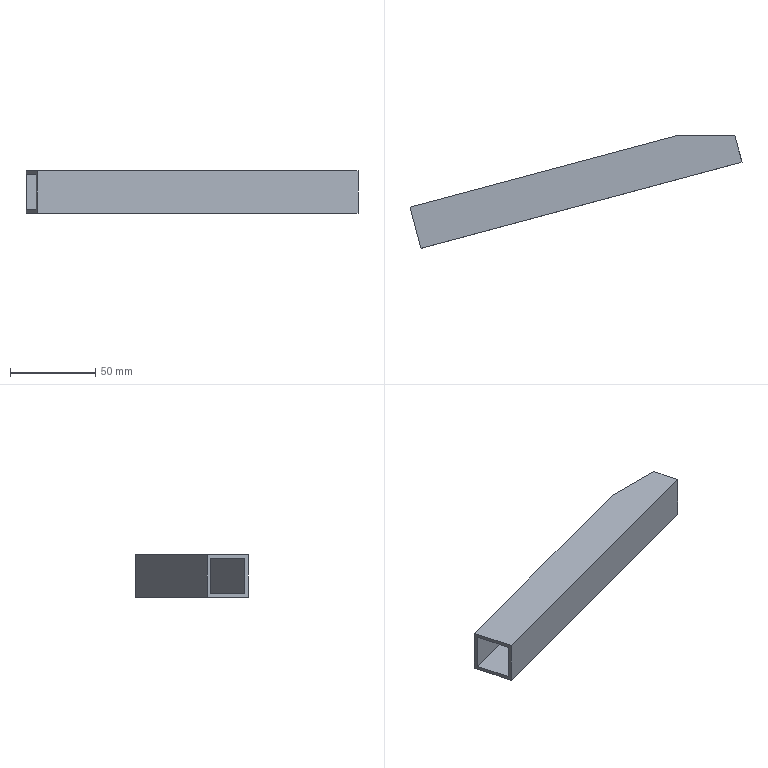Part | NX | features solid 2 | 1 solid | 11 faces | box 194.826 x 66.03 x 25 mm | volume 34053 mm3 | plane 11
STEP:
#1=CARTESIAN_POINT('',(-803.04,-87.5,-30.));
#2=VERTEX_POINT('',#1);
#3=CARTESIAN_POINT('',(-798.87,-103.06,-30.));
#4=VERTEX_POINT('',#3);
#5=CARTESIAN_POINT('',(-805.341,-78.912,-30.));
#6=DIRECTION('',(-0.2588,0.9659,0.));
#7=VECTOR('',#6,1000.);
#8=LINE('',#5,#7);
#9=EDGE_CURVE('',#2,#4,#8,.F.);
#10=ORIENTED_EDGE('',*,*,#9,.F.);
#11=CARTESIAN_POINT('',(-803.04,-87.5,-28.));
#12=VERTEX_POINT('',#11);
#13=CARTESIAN_POINT('',(-803.04,-87.5,-30.));
#14=DIRECTION('',(0.,0.,-1.));
#15=VECTOR('',#14,1000.);
#16=LINE('',#13,#15);
#17=EDGE_CURVE('',#2,#12,#16,.F.);
#18=ORIENTED_EDGE('',*,*,#17,.T.);
#19=CARTESIAN_POINT('',(-799.388,-101.128,-28.));
#20=VERTEX_POINT('',#19);
#21=CARTESIAN_POINT('',(-805.341,-78.912,-28.));
#22=DIRECTION('',(0.2588,-0.9659,0.));
#23=VECTOR('',#22,1000.);
#24=LINE('',#21,#23);
#25=EDGE_CURVE('',#12,#20,#24,.T.);
#26=ORIENTED_EDGE('',*,*,#25,.T.);
#27=CARTESIAN_POINT('',(-799.388,-101.128,-7.));
#28=VERTEX_POINT('',#27);
#29=CARTESIAN_POINT('',(-799.388,-101.128,-30.));
#30=DIRECTION('',(0.,0.,1.));
#31=VECTOR('',#30,1000.);
#32=LINE('',#29,#31);
#33=EDGE_CURVE('',#20,#28,#32,.T.);
#34=ORIENTED_EDGE('',*,*,#33,.T.);
#35=CARTESIAN_POINT('',(-803.04,-87.5,-7.));
#36=VERTEX_POINT('',#35);
#37=CARTESIAN_POINT('',(-805.341,-78.912,-7.));
#38=DIRECTION('',(0.2588,-0.9659,0.));
#39=VECTOR('',#38,1000.);
#40=LINE('',#37,#39);
#41=EDGE_CURVE('',#36,#28,#40,.T.);
#42=ORIENTED_EDGE('',*,*,#41,.F.);
#43=CARTESIAN_POINT('',(-803.04,-87.5,-5.));
#44=VERTEX_POINT('',#43);
#45=CARTESIAN_POINT('',(-803.04,-87.5,-30.));
#46=DIRECTION('',(0.,0.,-1.));
#47=VECTOR('',#46,1000.);
#48=LINE('',#45,#47);
#49=EDGE_CURVE('',#36,#44,#48,.F.);
#50=ORIENTED_EDGE('',*,*,#49,.T.);
#51=CARTESIAN_POINT('',(-798.87,-103.06,-5.));
#52=VERTEX_POINT('',#51);
#53=CARTESIAN_POINT('',(-805.341,-78.912,-5.));
#54=DIRECTION('',(0.2588,-0.9659,0.));
#55=VECTOR('',#54,1000.);
#56=LINE('',#53,#55);
#57=EDGE_CURVE('',#44,#52,#56,.T.);
#58=ORIENTED_EDGE('',*,*,#57,.T.);
#59=CARTESIAN_POINT('',(-798.87,-103.06,-30.));
#60=DIRECTION('',(0.,0.,-1.));
#61=VECTOR('',#60,1000.);
#62=LINE('',#59,#61);
#63=EDGE_CURVE('',#4,#52,#62,.F.);
#64=ORIENTED_EDGE('',*,*,#63,.F.);
#65=EDGE_LOOP('',(#10,#18,#26,#34,#42,#50,#58,#64));
#66=FACE_BOUND('',#65,.T.);
#67=CARTESIAN_POINT('',(-805.341,-78.912,-30.));
#68=DIRECTION('',(-0.9659,-0.2588,0.));
#69=DIRECTION('',(0.,0.,1.));
#70=AXIS2_PLACEMENT_3D('',#67,#68,#69);
#71=PLANE('',#70);
#72=ADVANCED_FACE('',(#66),#71,.F.);
#73=CARTESIAN_POINT('',(-993.696,-129.382,-5.));
#74=VERTEX_POINT('',#73);
#75=CARTESIAN_POINT('',(-987.226,-153.53,-5.));
#76=VERTEX_POINT('',#75);
#77=CARTESIAN_POINT('',(-993.696,-129.382,-5.));
#78=DIRECTION('',(0.2588,-0.9659,0.));
#79=VECTOR('',#78,1000.);
#80=LINE('',#77,#79);
#81=EDGE_CURVE('',#74,#76,#80,.T.);
#82=ORIENTED_EDGE('',*,*,#81,.F.);
#83=CARTESIAN_POINT('',(-993.696,-129.382,-30.));
#84=VERTEX_POINT('',#83);
#85=CARTESIAN_POINT('',(-993.696,-129.382,-30.));
#86=DIRECTION('',(0.,0.,1.));
#87=VECTOR('',#86,1000.);
#88=LINE('',#85,#87);
#89=EDGE_CURVE('',#84,#74,#88,.T.);
#90=ORIENTED_EDGE('',*,*,#89,.F.);
#91=CARTESIAN_POINT('',(-987.226,-153.53,-30.));
#92=VERTEX_POINT('',#91);
#93=CARTESIAN_POINT('',(-993.696,-129.382,-30.));
#94=DIRECTION('',(-0.2588,0.9659,0.));
#95=VECTOR('',#94,1000.);
#96=LINE('',#93,#95);
#97=EDGE_CURVE('',#84,#92,#96,.F.);
#98=ORIENTED_EDGE('',*,*,#97,.T.);
#99=CARTESIAN_POINT('',(-987.226,-153.53,-30.));
#100=DIRECTION('',(0.,0.,-1.));
#101=VECTOR('',#100,1000.);
#102=LINE('',#99,#101);
#103=EDGE_CURVE('',#92,#76,#102,.F.);
#104=ORIENTED_EDGE('',*,*,#103,.T.);
#105=EDGE_LOOP('',(#82,#90,#98,#104));
#106=FACE_BOUND('',#105,.T.);
#107=CARTESIAN_POINT('',(-993.179,-131.313,-28.));
#108=VERTEX_POINT('',#107);
#109=CARTESIAN_POINT('',(-993.179,-131.313,-7.));
#110=VERTEX_POINT('',#109);
#111=CARTESIAN_POINT('',(-993.179,-131.313,-30.));
#112=DIRECTION('',(0.,0.,1.));
#113=VECTOR('',#112,1000.);
#114=LINE('',#111,#113);
#115=EDGE_CURVE('',#108,#110,#114,.T.);
#116=ORIENTED_EDGE('',*,*,#115,.T.);
#117=CARTESIAN_POINT('',(-987.743,-151.598,-7.));
#118=VERTEX_POINT('',#117);
#119=CARTESIAN_POINT('',(-993.696,-129.382,-7.));
#120=DIRECTION('',(0.2588,-0.9659,0.));
#121=VECTOR('',#120,1000.);
#122=LINE('',#119,#121);
#123=EDGE_CURVE('',#110,#118,#122,.T.);
#124=ORIENTED_EDGE('',*,*,#123,.T.);
#125=CARTESIAN_POINT('',(-987.743,-151.598,-28.));
#126=VERTEX_POINT('',#125);
#127=CARTESIAN_POINT('',(-987.743,-151.598,-30.));
#128=DIRECTION('',(0.,0.,-1.));
#129=VECTOR('',#128,1000.);
#130=LINE('',#127,#129);
#131=EDGE_CURVE('',#126,#118,#130,.F.);
#132=ORIENTED_EDGE('',*,*,#131,.F.);
#133=CARTESIAN_POINT('',(-993.696,-129.382,-28.));
#134=DIRECTION('',(-0.2588,0.9659,0.));
#135=VECTOR('',#134,1000.);
#136=LINE('',#133,#135);
#137=EDGE_CURVE('',#108,#126,#136,.F.);
#138=ORIENTED_EDGE('',*,*,#137,.F.);
#139=EDGE_LOOP('',(#116,#124,#132,#138));
#140=FACE_BOUND('',#139,.T.);
#141=CARTESIAN_POINT('',(-993.696,-129.382,-30.));
#142=DIRECTION('',(-0.9659,-0.2588,0.));
#143=DIRECTION('',(0.,0.,1.));
#144=AXIS2_PLACEMENT_3D('',#141,#142,#143);
#145=PLANE('',#144);
#146=ADVANCED_FACE('',(#106,#140),#145,.T.);
#147=CARTESIAN_POINT('',(-837.392,-87.5,-30.));
#148=VERTEX_POINT('',#147);
#149=CARTESIAN_POINT('',(-839.148,-87.97,-30.));
#150=DIRECTION('',(-0.9659,-0.2588,0.));
#151=VECTOR('',#150,1000.);
#152=LINE('',#149,#151);
#153=EDGE_CURVE('',#84,#148,#152,.F.);
#154=ORIENTED_EDGE('',*,*,#153,.T.);
#155=CARTESIAN_POINT('',(-839.148,-87.5,-30.));
#156=DIRECTION('',(1.,0.,0.));
#157=VECTOR('',#156,1000.);
#158=LINE('',#155,#157);
#159=EDGE_CURVE('',#148,#2,#158,.T.);
#160=ORIENTED_EDGE('',*,*,#159,.T.);
#161=ORIENTED_EDGE('',*,*,#9,.T.);
#162=CARTESIAN_POINT('',(-832.678,-112.119,-30.));
#163=DIRECTION('',(-0.9659,-0.2588,0.));
#164=VECTOR('',#163,1000.);
#165=LINE('',#162,#164);
#166=EDGE_CURVE('',#92,#4,#165,.F.);
#167=ORIENTED_EDGE('',*,*,#166,.F.);
#168=ORIENTED_EDGE('',*,*,#97,.F.);
#169=EDGE_LOOP('',(#154,#160,#161,#167,#168));
#170=FACE_BOUND('',#169,.T.);
#171=CARTESIAN_POINT('',(-839.148,-87.97,-30.));
#172=DIRECTION('',(0.,0.,-1.));
#173=DIRECTION('',(0.2588,-0.9659,0.));
#174=AXIS2_PLACEMENT_3D('',#171,#172,#173);
#175=PLANE('',#174);
#176=ADVANCED_FACE('',(#170),#175,.T.);
#177=ORIENTED_EDGE('',*,*,#166,.T.);
#178=ORIENTED_EDGE('',*,*,#63,.T.);
#179=CARTESIAN_POINT('',(-832.678,-112.119,-5.));
#180=DIRECTION('',(-0.9659,-0.2588,0.));
#181=VECTOR('',#180,1000.);
#182=LINE('',#179,#181);
#183=EDGE_CURVE('',#76,#52,#182,.F.);
#184=ORIENTED_EDGE('',*,*,#183,.F.);
#185=ORIENTED_EDGE('',*,*,#103,.F.);
#186=EDGE_LOOP('',(#177,#178,#184,#185));
#187=FACE_BOUND('',#186,.T.);
#188=CARTESIAN_POINT('',(-832.678,-112.119,-30.));
#189=DIRECTION('',(0.2588,-0.9659,0.));
#190=DIRECTION('',(0.,0.,1.));
#191=AXIS2_PLACEMENT_3D('',#188,#189,#190);
#192=PLANE('',#191);
#193=ADVANCED_FACE('',(#187),#192,.T.);
#194=ORIENTED_EDGE('',*,*,#57,.F.);
#195=CARTESIAN_POINT('',(-837.392,-87.5,-5.));
#196=VERTEX_POINT('',#195);
#197=CARTESIAN_POINT('',(-839.148,-87.5,-5.));
#198=DIRECTION('',(1.,0.,0.));
#199=VECTOR('',#198,1000.);
#200=LINE('',#197,#199);
#201=EDGE_CURVE('',#44,#196,#200,.F.);
#202=ORIENTED_EDGE('',*,*,#201,.T.);
#203=CARTESIAN_POINT('',(-839.148,-87.97,-5.));
#204=DIRECTION('',(-0.9659,-0.2588,0.));
#205=VECTOR('',#204,1000.);
#206=LINE('',#203,#205);
#207=EDGE_CURVE('',#74,#196,#206,.F.);
#208=ORIENTED_EDGE('',*,*,#207,.F.);
#209=ORIENTED_EDGE('',*,*,#81,.T.);
#210=ORIENTED_EDGE('',*,*,#183,.T.);
#211=EDGE_LOOP('',(#194,#202,#208,#209,#210));
#212=FACE_BOUND('',#211,.T.);
#213=CARTESIAN_POINT('',(-839.148,-87.97,-5.));
#214=DIRECTION('',(0.,0.,-1.));
#215=DIRECTION('',(0.2588,-0.9659,0.));
#216=AXIS2_PLACEMENT_3D('',#213,#214,#215);
#217=PLANE('',#216);
#218=ADVANCED_FACE('',(#212),#217,.F.);
#219=ORIENTED_EDGE('',*,*,#207,.T.);
#220=CARTESIAN_POINT('',(-837.392,-87.5,-30.));
#221=DIRECTION('',(0.,0.,1.));
#222=VECTOR('',#221,1000.);
#223=LINE('',#220,#222);
#224=EDGE_CURVE('',#196,#148,#223,.F.);
#225=ORIENTED_EDGE('',*,*,#224,.T.);
#226=ORIENTED_EDGE('',*,*,#153,.F.);
#227=ORIENTED_EDGE('',*,*,#89,.T.);
#228=EDGE_LOOP('',(#219,#225,#226,#227));
#229=FACE_BOUND('',#228,.T.);
#230=CARTESIAN_POINT('',(-839.148,-87.97,-30.));
#231=DIRECTION('',(0.2588,-0.9659,0.));
#232=DIRECTION('',(0.,0.,1.));
#233=AXIS2_PLACEMENT_3D('',#230,#231,#232);
#234=PLANE('',#233);
#235=ADVANCED_FACE('',(#229),#234,.F.);
#236=CARTESIAN_POINT('',(-829.665,-87.5,-28.));
#237=VERTEX_POINT('',#236);
#238=CARTESIAN_POINT('',(-839.148,-87.5,-28.));
#239=DIRECTION('',(1.,0.,0.));
#240=VECTOR('',#239,1000.);
#241=LINE('',#238,#240);
#242=EDGE_CURVE('',#237,#12,#241,.T.);
#243=ORIENTED_EDGE('',*,*,#242,.F.);
#244=CARTESIAN_POINT('',(-838.631,-89.902,-28.));
#245=DIRECTION('',(-0.9659,-0.2588,0.));
#246=VECTOR('',#245,1000.);
#247=LINE('',#244,#246);
#248=EDGE_CURVE('',#108,#237,#247,.F.);
#249=ORIENTED_EDGE('',*,*,#248,.F.);
#250=ORIENTED_EDGE('',*,*,#137,.T.);
#251=CARTESIAN_POINT('',(-833.195,-110.187,-28.));
#252=DIRECTION('',(0.9659,0.2588,0.));
#253=VECTOR('',#252,1000.);
#254=LINE('',#251,#253);
#255=EDGE_CURVE('',#126,#20,#254,.T.);
#256=ORIENTED_EDGE('',*,*,#255,.T.);
#257=ORIENTED_EDGE('',*,*,#25,.F.);
#258=EDGE_LOOP('',(#243,#249,#250,#256,#257));
#259=FACE_BOUND('',#258,.T.);
#260=CARTESIAN_POINT('',(-839.148,-87.97,-28.));
#261=DIRECTION('',(0.,0.,-1.));
#262=DIRECTION('',(0.2588,-0.9659,0.));
#263=AXIS2_PLACEMENT_3D('',#260,#261,#262);
#264=PLANE('',#263);
#265=ADVANCED_FACE('',(#259),#264,.F.);
#266=ORIENTED_EDGE('',*,*,#255,.F.);
#267=ORIENTED_EDGE('',*,*,#131,.T.);
#268=CARTESIAN_POINT('',(-833.195,-110.187,-7.));
#269=DIRECTION('',(-0.9659,-0.2588,0.));
#270=VECTOR('',#269,1000.);
#271=LINE('',#268,#270);
#272=EDGE_CURVE('',#118,#28,#271,.F.);
#273=ORIENTED_EDGE('',*,*,#272,.T.);
#274=ORIENTED_EDGE('',*,*,#33,.F.);
#275=EDGE_LOOP('',(#266,#267,#273,#274));
#276=FACE_BOUND('',#275,.T.);
#277=CARTESIAN_POINT('',(-833.195,-110.187,-30.));
#278=DIRECTION('',(0.2588,-0.9659,0.));
#279=DIRECTION('',(0.,0.,1.));
#280=AXIS2_PLACEMENT_3D('',#277,#278,#279);
#281=PLANE('',#280);
#282=ADVANCED_FACE('',(#276),#281,.F.);
#283=CARTESIAN_POINT('',(-829.665,-87.5,-7.));
#284=VERTEX_POINT('',#283);
#285=CARTESIAN_POINT('',(-839.148,-87.5,-7.));
#286=DIRECTION('',(1.,0.,0.));
#287=VECTOR('',#286,1000.);
#288=LINE('',#285,#287);
#289=EDGE_CURVE('',#36,#284,#288,.F.);
#290=ORIENTED_EDGE('',*,*,#289,.F.);
#291=ORIENTED_EDGE('',*,*,#41,.T.);
#292=ORIENTED_EDGE('',*,*,#272,.F.);
#293=ORIENTED_EDGE('',*,*,#123,.F.);
#294=CARTESIAN_POINT('',(-838.631,-89.902,-7.));
#295=DIRECTION('',(0.9659,0.2588,0.));
#296=VECTOR('',#295,1000.);
#297=LINE('',#294,#296);
#298=EDGE_CURVE('',#110,#284,#297,.T.);
#299=ORIENTED_EDGE('',*,*,#298,.T.);
#300=EDGE_LOOP('',(#290,#291,#292,#293,#299));
#301=FACE_BOUND('',#300,.T.);
#302=CARTESIAN_POINT('',(-839.148,-87.97,-7.));
#303=DIRECTION('',(0.,0.,-1.));
#304=DIRECTION('',(0.2588,-0.9659,0.));
#305=AXIS2_PLACEMENT_3D('',#302,#303,#304);
#306=PLANE('',#305);
#307=ADVANCED_FACE('',(#301),#306,.T.);
#308=CARTESIAN_POINT('',(-829.665,-87.5,-30.));
#309=DIRECTION('',(0.,0.,1.));
#310=VECTOR('',#309,1000.);
#311=LINE('',#308,#310);
#312=EDGE_CURVE('',#284,#237,#311,.F.);
#313=ORIENTED_EDGE('',*,*,#312,.F.);
#314=ORIENTED_EDGE('',*,*,#298,.F.);
#315=ORIENTED_EDGE('',*,*,#115,.F.);
#316=ORIENTED_EDGE('',*,*,#248,.T.);
#317=EDGE_LOOP('',(#313,#314,#315,#316));
#318=FACE_BOUND('',#317,.T.);
#319=CARTESIAN_POINT('',(-838.631,-89.902,-30.));
#320=DIRECTION('',(0.2588,-0.9659,0.));
#321=DIRECTION('',(0.,0.,1.));
#322=AXIS2_PLACEMENT_3D('',#319,#320,#321);
#323=PLANE('',#322);
#324=ADVANCED_FACE('',(#318),#323,.T.);
#325=ORIENTED_EDGE('',*,*,#201,.F.);
#326=ORIENTED_EDGE('',*,*,#49,.F.);
#327=ORIENTED_EDGE('',*,*,#289,.T.);
#328=ORIENTED_EDGE('',*,*,#312,.T.);
#329=ORIENTED_EDGE('',*,*,#242,.T.);
#330=ORIENTED_EDGE('',*,*,#17,.F.);
#331=ORIENTED_EDGE('',*,*,#159,.F.);
#332=ORIENTED_EDGE('',*,*,#224,.F.);
#333=EDGE_LOOP('',(#325,#326,#327,#328,#329,#330,#331,#332));
#334=FACE_BOUND('',#333,.T.);
#335=CARTESIAN_POINT('',(-690.,-87.5,-55.));
#336=DIRECTION('',(0.,1.,0.));
#337=DIRECTION('',(1.,0.,0.));
#338=AXIS2_PLACEMENT_3D('',#335,#336,#337);
#339=PLANE('',#338);
#340=ADVANCED_FACE('',(#334),#339,.T.);
#341=CLOSED_SHELL('',(#72,#146,#176,#193,#218,#235,#265,#282,#307,#324,#340));
#342=MANIFOLD_SOLID_BREP('',#341);
#343=(LENGTH_UNIT()NAMED_UNIT(*)SI_UNIT(.MILLI.,.METRE.));
#344=UNCERTAINTY_MEASURE_WITH_UNIT(LENGTH_MEASURE(0.00001),#343,'','');
#345=(NAMED_UNIT(*)PLANE_ANGLE_UNIT()SI_UNIT($,.RADIAN.));
#346=(NAMED_UNIT(*)SI_UNIT($,.STERADIAN.)SOLID_ANGLE_UNIT());
#347=(GEOMETRIC_REPRESENTATION_CONTEXT(3)GLOBAL_UNCERTAINTY_ASSIGNED_CONTEXT((#344))GLOBAL_UNIT_ASSIGNED_CONTEXT((#343,#345,#346))REPRESENTATION_CONTEXT('',''));
#348=ADVANCED_BREP_SHAPE_REPRESENTATION('',(#342),#347);